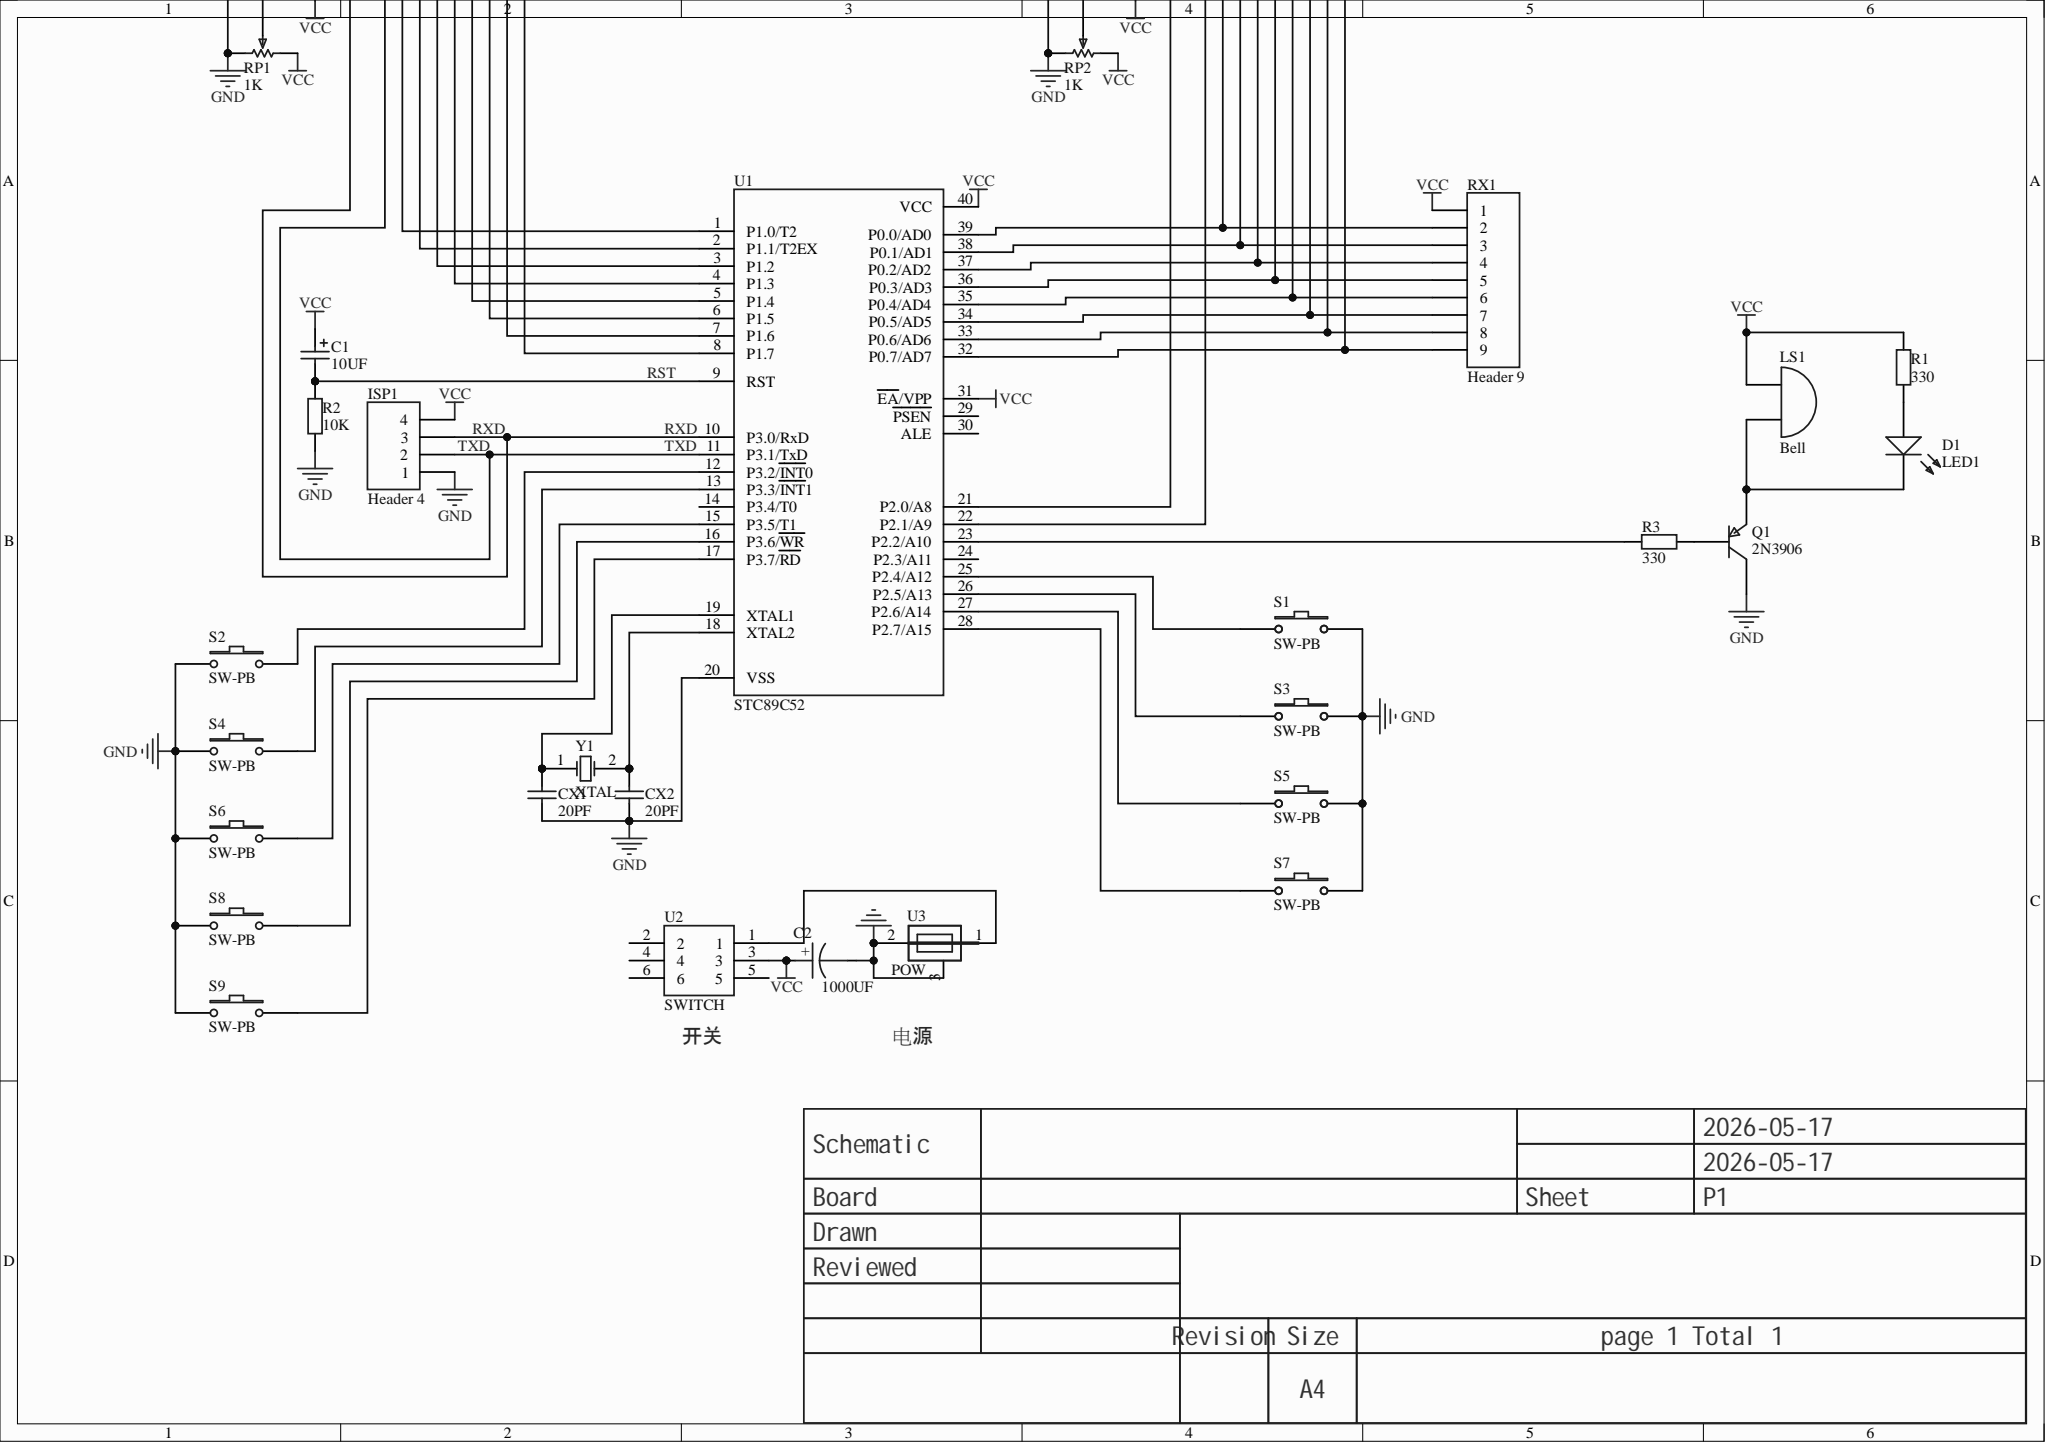Circuit board | Altium Designer | 29 parts | 41 nets
Bill of materials:
Comment,Description,Designator,Footprint,LibRef,Quantity
"Cap Pol2","Polarized Capacitor (Axial)","C1","CAP-TH_BD5.0-P2.00-D0.8-FD-10UF50VC110GL","Cap Pol2","1"
"1000UF","","C2","CAP-TH_BD5.0-P2.00-D0.8-FD-10UF50VC110GL","10uF","1"
"Cap","Capacitor","CX1, CX2","CAP-TH_L5.0-W2.5-P5.00-D1.0","Cap","2"
"LED1","Typical RED GaAs LED","D1","LED_TH-3mm","LED1","1"
"Header 4","Header, 4-Pin","ISP1","HDR-TH_4P-P2.54-V-F","Header 4","1"
"1602","","LCD1, LCD2","LCD1602","1602","2"
"Bell","Electrical Bell","LS1","BUZ-TH_BD12.0-P6.00-D0.9-RD","Bell","1"
"2N3906","PNP General Purpose Amplifier","Q1","TO-92-3_L4.6-W3.6-P1.27-L_1","2N3906","1"
"Res2","Resistor","R1, R2, R3","Res_1/8W","Res2, Res2_1","3"
"RPot","Potentiometer","RP1, RP2","RES-ADJ-SMD_RM065-V1","RPot_1, RPot","2"
"Header 9","Header, 9-Pin","RX1","HDR-TH_9P-P2.54-V-F-1","Header 9","1"
"SW-PB","Switch","S1, S2, S3, S4, S5, S6, S7, S8, S9","SW-TH_4P-L6.0-W6.0-P4.50-LS6.5","SW-PB, SW-PB_1","9"
"STC89C52","","U1","DIP-40_L52.0-W13.7-P2.54-LS15.2-BL","AT89C51","1"
"SWITCH","","U2","SW-TH_6P-L5.8-W5.8-P2.00-LS4.5-BL","SWITCH","1"
"POW","","U3","DC-IN-TH_DC005","POW","1"
"XTAL","Crystal Oscillator","Y1","HC-49S_L11.5-W5.0-P4.88","XTAL","1"
Netlist (Protel format):
[
C1
CAP-TH_BD5.0-P2.00-D0.8-FD-10UF50VC110GL
Cap Pol2



]
[
C2
CAP-TH_BD5.0-P2.00-D0.8-FD-10UF50VC110GL
1000UF



]
[
CX1
CAP-TH_L5.0-W2.5-P5.00-D1.0
Cap



]
[
CX2
CAP-TH_L5.0-W2.5-P5.00-D1.0
Cap



]
[
D1
LED_TH-3mm
LED1



]
[
ISP1
HDR-TH_4P-P2.54-V-F
Header 4



]
[
LCD1
LCD1602
1602



]
[
LCD2
LCD1602
1602



]
[
LS1
BUZ-TH_BD12.0-P6.00-D0.9-RD
Bell



]
[
Q1
TO-92-3_L4.6-W3.6-P1.27-L_1
2N3906



]
[
R1
Res_1/8W
Res2



]
[
R2
Res_1/8W
Res2



]
[
R3
Res_1/8W
Res2



]
[
RP1
RES-ADJ-SMD_RM065-V1
RPot



]
[
RP2
RES-ADJ-SMD_RM065-V1
RPot



]
[
RX1
HDR-TH_9P-P2.54-V-F-1
Header 9



]
[
S1
SW-TH_4P-L6.0-W6.0-P4.50-LS6.5
SW-PB



]
[
S2
SW-TH_4P-L6.0-W6.0-P4.50-LS6.5
SW-PB



]
[
S3
SW-TH_4P-L6.0-W6.0-P4.50-LS6.5
SW-PB



]
[
S4
SW-TH_4P-L6.0-W6.0-P4.50-LS6.5
SW-PB



]
[
S5
SW-TH_4P-L6.0-W6.0-P4.50-LS6.5
SW-PB



]
[
S6
SW-TH_4P-L6.0-W6.0-P4.50-LS6.5
SW-PB



]
[
S7
SW-TH_4P-L6.0-W6.0-P4.50-LS6.5
SW-PB



]
[
S8
SW-TH_4P-L6.0-W6.0-P4.50-LS6.5
SW-PB



]
[
S9
SW-TH_4P-L6.0-W6.0-P4.50-LS6.5
SW-PB



]
[
U1
DIP-40_L52.0-W13.7-P2.54-LS15.2-BL
STC89C52



]
[
U2
SW-TH_6P-L5.8-W5.8-P2.00-LS4.5-BL
SWITCH



]
[
U3
DC-IN-TH_DC005
POW



]
[
Y1
HC-49S_L11.5-W5.0-P4.88
XTAL



]
(
VCC
C1-1
C2-1
ISP1-4
LCD1-2
LCD1-15
LCD2-2
LCD2-15
LS1-1
R1-2
RP1-1
RP2-1
RX1-1
U1-31
U1-40
U2-3
)
(
TXD
ISP1-2
LCD1-6
U1-11
)
(
RXD
ISP1-3
LCD1-4
U1-10
)
(
RST
C1-2
R2-2
U1-9
)
(
NetU2_1
U2-1
U3-1
)
(
NetS9_1
S9-1
U1-17
)
(
NetS8_1
S8-1
U1-16
)
(
NetS7_1
S7-1
U1-28
)
(
NetS6_1
S6-1
U1-15
)
(
NetS5_1
S5-1
U1-27
)
(
NetS4_1
S4-1
U1-13
)
(
NetS3_1
S3-1
U1-26
)
(
NetS2_1
S2-1
U1-12
)
(
NetS1_1
S1-1
U1-25
)
(
NetR3_1
R3-1
U1-23
)
(
NetQ1_2
Q1-2
R3-2
)
(
NetLCD2_14
LCD2-14
RX1-9
U1-32
)
(
NetLCD2_13
LCD2-13
RX1-8
U1-33
)
(
NetLCD2_12
LCD2-12
RX1-7
U1-34
)
(
NetLCD2_11
LCD2-11
RX1-6
U1-35
)
(
NetLCD2_10
LCD2-10
RX1-5
U1-36
)
(
NetLCD2_9
LCD2-9
RX1-4
U1-37
)
(
NetLCD2_8
LCD2-8
RX1-3
U1-38
)
(
NetLCD2_7
LCD2-7
RX1-2
U1-39
)
(
NetLCD2_6
LCD2-6
U1-22
)
(
NetLCD2_4
LCD2-4
U1-21
)
(
NetLCD2_3
LCD2-3
RP2-3
)
(
NetLCD1_14
LCD1-14
U1-8
)
(
NetLCD1_13
LCD1-13
U1-7
)
(
NetLCD1_12
LCD1-12
U1-6
)
(
NetLCD1_11
LCD1-11
U1-5
)
(
NetLCD1_10
LCD1-10
U1-4
)
(
NetLCD1_9
LCD1-9
U1-3
)
(
NetLCD1_8
LCD1-8
U1-2
)
(
NetLCD1_7
LCD1-7
U1-1
)
(
NetLCD1_3
LCD1-3
RP1-3
)
(
NetD1_2
D1-2
LS1-2
Q1-1
)
(
NetD1_1
D1-1
R1-1
)
(
NetCX2_2
CX2-2
U1-18
Y1-2
)
(
NetCX1_2
CX1-2
U1-19
Y1-1
)
(
GND
C2-2
CX1-1
CX2-1
ISP1-1
LCD1-1
LCD1-5
LCD1-16
LCD2-1
LCD2-5
LCD2-16
Q1-3
R2-1
RP1-2
RP2-2
S1-2
S2-2
S3-2
S4-2
S5-2
S6-2
S7-2
S8-2
S9-2
U1-20
U3-2
U3-3
)